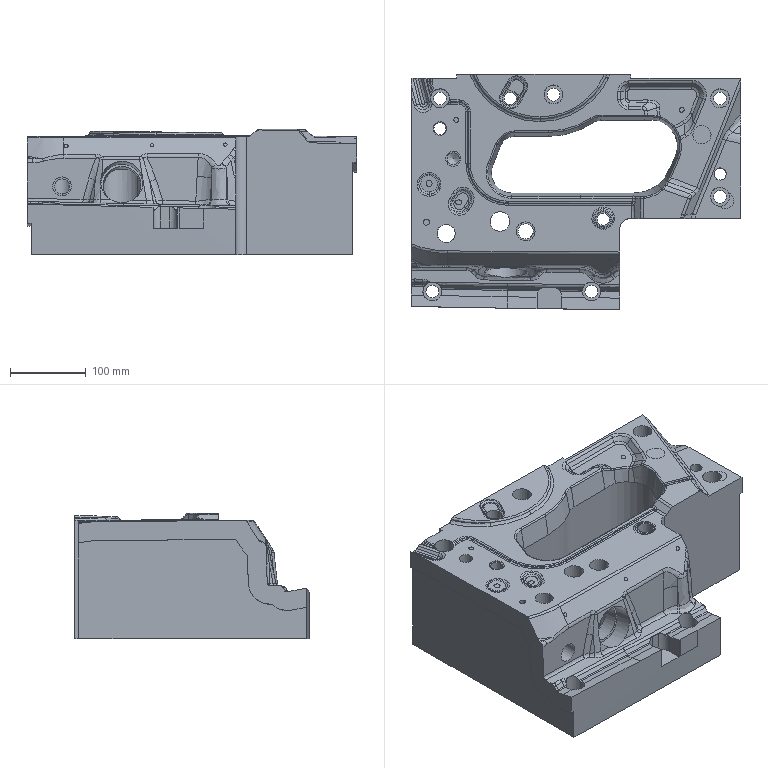Part | NX | features solid 2 | 1 solid | 408 faces | box 438.042 x 310.072 x 165.822 mm | volume 11649735 mm3 | spline 333 | cylinder 38 | plane 36 | cone 1 | commonest cylinder face diameters 25 x8 20 x7 17 x6 16 x5 23 x2 52 x2